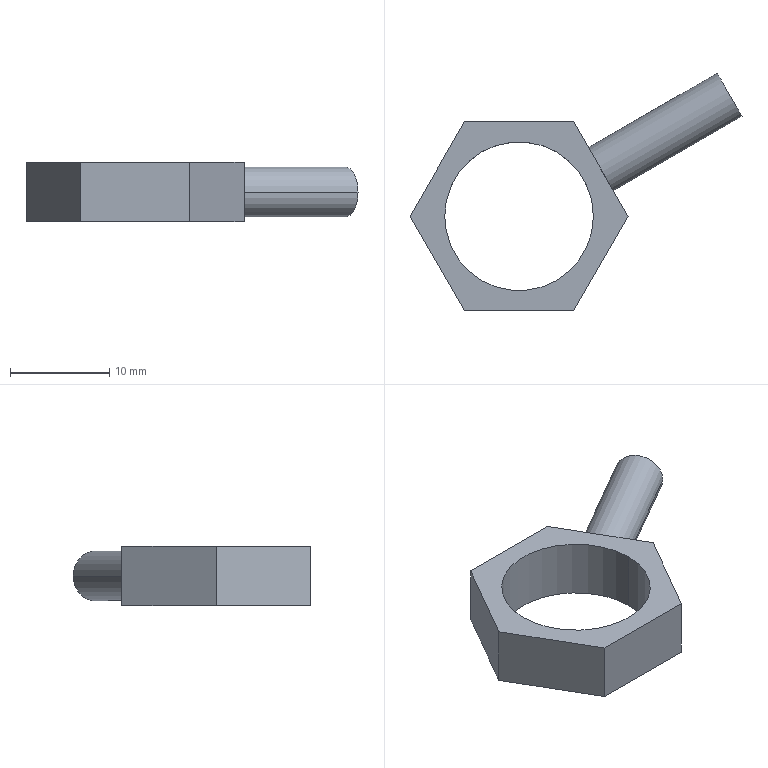Part | SolidWorks | features Extrusion 1, ICE 1 | 1 solid | 13 faces | box 33.49 x 23.954 x 6 mm | volume 1120 mm3 | plane 9 | cylinder 4 | commonest cylinder face diameters 5 x2 15 x2
STEP:
#1=CARTESIAN_POINT('',(19.99,14.428,3.));
#2=VERTEX_POINT('',#1);
#3=CARTESIAN_POINT('',(22.49,10.098,3.));
#4=VERTEX_POINT('',#3);
#5=CARTESIAN_POINT('',(21.24,12.263,3.));
#6=DIRECTION('',(0.866,0.5,0.));
#7=DIRECTION('',(-0.5,0.866,0.));
#8=AXIS2_PLACEMENT_3D('',#5,#6,#7);
#9=CIRCLE('',#8,2.5);
#10=EDGE_CURVE('',#2,#4,#9,.T.);
#11=ORIENTED_EDGE('',*,*,#10,.F.);
#12=CARTESIAN_POINT('',(7.,6.928,3.));
#13=VERTEX_POINT('',#12);
#14=CARTESIAN_POINT('',(19.99,14.428,3.));
#15=DIRECTION('',(-0.866,-0.5,0.));
#16=VECTOR('',#15,1000.);
#17=LINE('',#14,#16);
#18=EDGE_CURVE('',#2,#13,#17,.T.);
#19=ORIENTED_EDGE('',*,*,#18,.T.);
#20=CARTESIAN_POINT('',(9.5,2.598,3.));
#21=VERTEX_POINT('',#20);
#22=CARTESIAN_POINT('',(8.25,4.763,3.));
#23=DIRECTION('',(0.866,0.5,0.));
#24=DIRECTION('',(-0.5,0.866,0.));
#25=AXIS2_PLACEMENT_3D('',#22,#23,#24);
#26=CIRCLE('',#25,2.5);
#27=EDGE_CURVE('',#13,#21,#26,.T.);
#28=ORIENTED_EDGE('',*,*,#27,.T.);
#29=CARTESIAN_POINT('',(22.49,10.098,3.));
#30=DIRECTION('',(-0.866,-0.5,0.));
#31=VECTOR('',#30,1000.);
#32=LINE('',#29,#31);
#33=EDGE_CURVE('',#4,#21,#32,.T.);
#34=ORIENTED_EDGE('',*,*,#33,.F.);
#35=EDGE_LOOP('',(#11,#19,#28,#34));
#36=FACE_OUTER_BOUND('',#35,.T.);
#37=CARTESIAN_POINT('',(21.24,12.263,3.));
#38=DIRECTION('',(-0.866,-0.5,0.));
#39=DIRECTION('',(0.5,-0.866,0.));
#40=AXIS2_PLACEMENT_3D('',#37,#38,#39);
#41=CYLINDRICAL_SURFACE('',#40,2.5);
#42=ADVANCED_FACE('',(#36),#41,.T.);
#43=CARTESIAN_POINT('',(-7.5,0.,6.));
#44=VERTEX_POINT('',#43);
#45=CARTESIAN_POINT('',(7.5,0.,6.));
#46=VERTEX_POINT('',#45);
#47=CARTESIAN_POINT('',(0.,0.,6.));
#48=DIRECTION('',(0.,0.,1.));
#49=DIRECTION('',(1.,0.,0.));
#50=AXIS2_PLACEMENT_3D('',#47,#48,#49);
#51=CIRCLE('',#50,7.5);
#52=EDGE_CURVE('',#44,#46,#51,.T.);
#53=ORIENTED_EDGE('',*,*,#52,.T.);
#54=CARTESIAN_POINT('',(7.5,0.,0.));
#55=VERTEX_POINT('',#54);
#56=CARTESIAN_POINT('',(7.5,0.,6.));
#57=DIRECTION('',(0.,0.,-1.));
#58=VECTOR('',#57,1000.);
#59=LINE('',#56,#58);
#60=EDGE_CURVE('',#46,#55,#59,.T.);
#61=ORIENTED_EDGE('',*,*,#60,.T.);
#62=CARTESIAN_POINT('',(-7.5,0.,0.));
#63=VERTEX_POINT('',#62);
#64=CARTESIAN_POINT('',(0.,0.,0.));
#65=DIRECTION('',(0.,0.,1.));
#66=DIRECTION('',(1.,0.,0.));
#67=AXIS2_PLACEMENT_3D('',#64,#65,#66);
#68=CIRCLE('',#67,7.5);
#69=EDGE_CURVE('',#63,#55,#68,.T.);
#70=ORIENTED_EDGE('',*,*,#69,.F.);
#71=CARTESIAN_POINT('',(-7.5,0.,6.));
#72=DIRECTION('',(0.,0.,-1.));
#73=VECTOR('',#72,1000.);
#74=LINE('',#71,#73);
#75=EDGE_CURVE('',#44,#63,#74,.T.);
#76=ORIENTED_EDGE('',*,*,#75,.F.);
#77=EDGE_LOOP('',(#53,#61,#70,#76));
#78=FACE_OUTER_BOUND('',#77,.T.);
#79=CARTESIAN_POINT('',(0.,0.,6.));
#80=DIRECTION('',(0.,0.,-1.));
#81=DIRECTION('',(-1.,0.,0.));
#82=AXIS2_PLACEMENT_3D('',#79,#80,#81);
#83=CYLINDRICAL_SURFACE('',#82,7.5);
#84=ADVANCED_FACE('',(#78),#83,.F.);
#85=CARTESIAN_POINT('',(5.5,9.526,6.));
#86=VERTEX_POINT('',#85);
#87=CARTESIAN_POINT('',(-5.5,9.526,6.));
#88=VERTEX_POINT('',#87);
#89=CARTESIAN_POINT('',(5.5,9.526,6.));
#90=DIRECTION('',(-1.,0.,0.));
#91=VECTOR('',#90,1000.);
#92=LINE('',#89,#91);
#93=EDGE_CURVE('',#86,#88,#92,.T.);
#94=ORIENTED_EDGE('',*,*,#93,.T.);
#95=CARTESIAN_POINT('',(-11.,0.,6.));
#96=VERTEX_POINT('',#95);
#97=CARTESIAN_POINT('',(-5.5,9.526,6.));
#98=DIRECTION('',(-0.5,-0.866,0.));
#99=VECTOR('',#98,1000.);
#100=LINE('',#97,#99);
#101=EDGE_CURVE('',#88,#96,#100,.T.);
#102=ORIENTED_EDGE('',*,*,#101,.T.);
#103=CARTESIAN_POINT('',(-5.5,-9.526,6.));
#104=VERTEX_POINT('',#103);
#105=CARTESIAN_POINT('',(-11.,0.,6.));
#106=DIRECTION('',(0.5,-0.866,0.));
#107=VECTOR('',#106,1000.);
#108=LINE('',#105,#107);
#109=EDGE_CURVE('',#96,#104,#108,.T.);
#110=ORIENTED_EDGE('',*,*,#109,.T.);
#111=CARTESIAN_POINT('',(5.5,-9.526,6.));
#112=VERTEX_POINT('',#111);
#113=CARTESIAN_POINT('',(-5.5,-9.526,6.));
#114=DIRECTION('',(1.,0.,0.));
#115=VECTOR('',#114,1000.);
#116=LINE('',#113,#115);
#117=EDGE_CURVE('',#104,#112,#116,.T.);
#118=ORIENTED_EDGE('',*,*,#117,.T.);
#119=CARTESIAN_POINT('',(11.,0.,6.));
#120=VERTEX_POINT('',#119);
#121=CARTESIAN_POINT('',(5.5,-9.526,6.));
#122=DIRECTION('',(0.5,0.866,0.));
#123=VECTOR('',#122,1000.);
#124=LINE('',#121,#123);
#125=EDGE_CURVE('',#112,#120,#124,.T.);
#126=ORIENTED_EDGE('',*,*,#125,.T.);
#127=CARTESIAN_POINT('',(11.,0.,6.));
#128=DIRECTION('',(-0.5,0.866,0.));
#129=VECTOR('',#128,1000.);
#130=LINE('',#127,#129);
#131=EDGE_CURVE('',#120,#86,#130,.T.);
#132=ORIENTED_EDGE('',*,*,#131,.T.);
#133=EDGE_LOOP('',(#94,#102,#110,#118,#126,#132));
#134=FACE_OUTER_BOUND('',#133,.T.);
#135=ORIENTED_EDGE('',*,*,#52,.F.);
#136=CARTESIAN_POINT('',(0.,0.,6.));
#137=DIRECTION('',(0.,0.,1.));
#138=DIRECTION('',(1.,0.,0.));
#139=AXIS2_PLACEMENT_3D('',#136,#137,#138);
#140=CIRCLE('',#139,7.5);
#141=EDGE_CURVE('',#46,#44,#140,.T.);
#142=ORIENTED_EDGE('',*,*,#141,.F.);
#143=EDGE_LOOP('',(#135,#142));
#144=FACE_BOUND('',#143,.T.);
#145=CARTESIAN_POINT('',(0.,0.,6.));
#146=DIRECTION('',(0.,0.,1.));
#147=DIRECTION('',(1.,0.,0.));
#148=AXIS2_PLACEMENT_3D('',#145,#146,#147);
#149=PLANE('',#148);
#150=ADVANCED_FACE('',(#134,#144),#149,.T.);
#151=CARTESIAN_POINT('',(5.5,9.526,0.));
#152=VERTEX_POINT('',#151);
#153=CARTESIAN_POINT('',(-5.5,9.526,0.));
#154=VERTEX_POINT('',#153);
#155=CARTESIAN_POINT('',(5.5,9.526,0.));
#156=DIRECTION('',(-1.,0.,0.));
#157=VECTOR('',#156,1000.);
#158=LINE('',#155,#157);
#159=EDGE_CURVE('',#152,#154,#158,.T.);
#160=ORIENTED_EDGE('',*,*,#159,.F.);
#161=CARTESIAN_POINT('',(11.,0.,0.));
#162=VERTEX_POINT('',#161);
#163=CARTESIAN_POINT('',(11.,0.,0.));
#164=DIRECTION('',(-0.5,0.866,0.));
#165=VECTOR('',#164,1000.);
#166=LINE('',#163,#165);
#167=EDGE_CURVE('',#162,#152,#166,.T.);
#168=ORIENTED_EDGE('',*,*,#167,.F.);
#169=CARTESIAN_POINT('',(5.5,-9.526,0.));
#170=VERTEX_POINT('',#169);
#171=CARTESIAN_POINT('',(5.5,-9.526,0.));
#172=DIRECTION('',(0.5,0.866,0.));
#173=VECTOR('',#172,1000.);
#174=LINE('',#171,#173);
#175=EDGE_CURVE('',#170,#162,#174,.T.);
#176=ORIENTED_EDGE('',*,*,#175,.F.);
#177=CARTESIAN_POINT('',(-5.5,-9.526,0.));
#178=VERTEX_POINT('',#177);
#179=CARTESIAN_POINT('',(-5.5,-9.526,0.));
#180=DIRECTION('',(1.,0.,0.));
#181=VECTOR('',#180,1000.);
#182=LINE('',#179,#181);
#183=EDGE_CURVE('',#178,#170,#182,.T.);
#184=ORIENTED_EDGE('',*,*,#183,.F.);
#185=CARTESIAN_POINT('',(-11.,0.,0.));
#186=VERTEX_POINT('',#185);
#187=CARTESIAN_POINT('',(-11.,0.,0.));
#188=DIRECTION('',(0.5,-0.866,0.));
#189=VECTOR('',#188,1000.);
#190=LINE('',#187,#189);
#191=EDGE_CURVE('',#186,#178,#190,.T.);
#192=ORIENTED_EDGE('',*,*,#191,.F.);
#193=CARTESIAN_POINT('',(-5.5,9.526,0.));
#194=DIRECTION('',(-0.5,-0.866,0.));
#195=VECTOR('',#194,1000.);
#196=LINE('',#193,#195);
#197=EDGE_CURVE('',#154,#186,#196,.T.);
#198=ORIENTED_EDGE('',*,*,#197,.F.);
#199=EDGE_LOOP('',(#160,#168,#176,#184,#192,#198));
#200=FACE_OUTER_BOUND('',#199,.T.);
#201=ORIENTED_EDGE('',*,*,#69,.T.);
#202=CARTESIAN_POINT('',(0.,0.,0.));
#203=DIRECTION('',(0.,0.,1.));
#204=DIRECTION('',(1.,0.,0.));
#205=AXIS2_PLACEMENT_3D('',#202,#203,#204);
#206=CIRCLE('',#205,7.5);
#207=EDGE_CURVE('',#55,#63,#206,.T.);
#208=ORIENTED_EDGE('',*,*,#207,.T.);
#209=EDGE_LOOP('',(#201,#208));
#210=FACE_BOUND('',#209,.T.);
#211=CARTESIAN_POINT('',(0.,0.,0.));
#212=DIRECTION('',(0.,0.,1.));
#213=DIRECTION('',(1.,0.,0.));
#214=AXIS2_PLACEMENT_3D('',#211,#212,#213);
#215=PLANE('',#214);
#216=ADVANCED_FACE('',(#200,#210),#215,.F.);
#217=ORIENTED_EDGE('',*,*,#159,.T.);
#218=CARTESIAN_POINT('',(-5.5,9.526,6.));
#219=DIRECTION('',(0.,0.,-1.));
#220=VECTOR('',#219,1000.);
#221=LINE('',#218,#220);
#222=EDGE_CURVE('',#88,#154,#221,.T.);
#223=ORIENTED_EDGE('',*,*,#222,.F.);
#224=ORIENTED_EDGE('',*,*,#93,.F.);
#225=CARTESIAN_POINT('',(5.5,9.526,6.));
#226=DIRECTION('',(0.,0.,-1.));
#227=VECTOR('',#226,1000.);
#228=LINE('',#225,#227);
#229=EDGE_CURVE('',#86,#152,#228,.T.);
#230=ORIENTED_EDGE('',*,*,#229,.T.);
#231=EDGE_LOOP('',(#217,#223,#224,#230));
#232=FACE_OUTER_BOUND('',#231,.T.);
#233=CARTESIAN_POINT('',(5.5,9.526,6.));
#234=DIRECTION('',(0.,-1.,0.));
#235=DIRECTION('',(1.,0.,0.));
#236=AXIS2_PLACEMENT_3D('',#233,#234,#235);
#237=PLANE('',#236);
#238=ADVANCED_FACE('',(#232),#237,.F.);
#239=ORIENTED_EDGE('',*,*,#197,.T.);
#240=CARTESIAN_POINT('',(-11.,0.,6.));
#241=DIRECTION('',(0.,0.,-1.));
#242=VECTOR('',#241,1000.);
#243=LINE('',#240,#242);
#244=EDGE_CURVE('',#96,#186,#243,.T.);
#245=ORIENTED_EDGE('',*,*,#244,.F.);
#246=ORIENTED_EDGE('',*,*,#101,.F.);
#247=ORIENTED_EDGE('',*,*,#222,.T.);
#248=EDGE_LOOP('',(#239,#245,#246,#247));
#249=FACE_OUTER_BOUND('',#248,.T.);
#250=CARTESIAN_POINT('',(-5.5,9.526,6.));
#251=DIRECTION('',(0.866,-0.5,0.));
#252=DIRECTION('',(0.5,0.866,0.));
#253=AXIS2_PLACEMENT_3D('',#250,#251,#252);
#254=PLANE('',#253);
#255=ADVANCED_FACE('',(#249),#254,.F.);
#256=ORIENTED_EDGE('',*,*,#191,.T.);
#257=CARTESIAN_POINT('',(-5.5,-9.526,6.));
#258=DIRECTION('',(0.,0.,-1.));
#259=VECTOR('',#258,1000.);
#260=LINE('',#257,#259);
#261=EDGE_CURVE('',#104,#178,#260,.T.);
#262=ORIENTED_EDGE('',*,*,#261,.F.);
#263=ORIENTED_EDGE('',*,*,#109,.F.);
#264=ORIENTED_EDGE('',*,*,#244,.T.);
#265=EDGE_LOOP('',(#256,#262,#263,#264));
#266=FACE_OUTER_BOUND('',#265,.T.);
#267=CARTESIAN_POINT('',(-11.,0.,6.));
#268=DIRECTION('',(0.866,0.5,0.));
#269=DIRECTION('',(-0.5,0.866,0.));
#270=AXIS2_PLACEMENT_3D('',#267,#268,#269);
#271=PLANE('',#270);
#272=ADVANCED_FACE('',(#266),#271,.F.);
#273=ORIENTED_EDGE('',*,*,#183,.T.);
#274=CARTESIAN_POINT('',(5.5,-9.526,6.));
#275=DIRECTION('',(0.,0.,-1.));
#276=VECTOR('',#275,1000.);
#277=LINE('',#274,#276);
#278=EDGE_CURVE('',#112,#170,#277,.T.);
#279=ORIENTED_EDGE('',*,*,#278,.F.);
#280=ORIENTED_EDGE('',*,*,#117,.F.);
#281=ORIENTED_EDGE('',*,*,#261,.T.);
#282=EDGE_LOOP('',(#273,#279,#280,#281));
#283=FACE_OUTER_BOUND('',#282,.T.);
#284=CARTESIAN_POINT('',(-5.5,-9.526,6.));
#285=DIRECTION('',(0.,1.,0.));
#286=DIRECTION('',(-1.,0.,0.));
#287=AXIS2_PLACEMENT_3D('',#284,#285,#286);
#288=PLANE('',#287);
#289=ADVANCED_FACE('',(#283),#288,.F.);
#290=ORIENTED_EDGE('',*,*,#175,.T.);
#291=CARTESIAN_POINT('',(11.,0.,6.));
#292=DIRECTION('',(0.,0.,-1.));
#293=VECTOR('',#292,1000.);
#294=LINE('',#291,#293);
#295=EDGE_CURVE('',#120,#162,#294,.T.);
#296=ORIENTED_EDGE('',*,*,#295,.F.);
#297=ORIENTED_EDGE('',*,*,#125,.F.);
#298=ORIENTED_EDGE('',*,*,#278,.T.);
#299=EDGE_LOOP('',(#290,#296,#297,#298));
#300=FACE_OUTER_BOUND('',#299,.T.);
#301=CARTESIAN_POINT('',(5.5,-9.526,6.));
#302=DIRECTION('',(-0.866,0.5,0.));
#303=DIRECTION('',(-0.5,-0.866,0.));
#304=AXIS2_PLACEMENT_3D('',#301,#302,#303);
#305=PLANE('',#304);
#306=ADVANCED_FACE('',(#300),#305,.F.);
#307=CARTESIAN_POINT('',(8.25,4.763,3.));
#308=DIRECTION('',(0.866,0.5,0.));
#309=DIRECTION('',(-0.5,0.866,0.));
#310=AXIS2_PLACEMENT_3D('',#307,#308,#309);
#311=CIRCLE('',#310,2.5);
#312=EDGE_CURVE('',#21,#13,#311,.T.);
#313=ORIENTED_EDGE('',*,*,#312,.F.);
#314=ORIENTED_EDGE('',*,*,#27,.F.);
#315=EDGE_LOOP('',(#313,#314));
#316=FACE_BOUND('',#315,.T.);
#317=ORIENTED_EDGE('',*,*,#167,.T.);
#318=ORIENTED_EDGE('',*,*,#229,.F.);
#319=ORIENTED_EDGE('',*,*,#131,.F.);
#320=ORIENTED_EDGE('',*,*,#295,.T.);
#321=EDGE_LOOP('',(#317,#318,#319,#320));
#322=FACE_OUTER_BOUND('',#321,.T.);
#323=CARTESIAN_POINT('',(11.,0.,6.));
#324=DIRECTION('',(-0.866,-0.5,0.));
#325=DIRECTION('',(0.5,-0.866,0.));
#326=AXIS2_PLACEMENT_3D('',#323,#324,#325);
#327=PLANE('',#326);
#328=ADVANCED_FACE('',(#316,#322),#327,.F.);
#329=ORIENTED_EDGE('',*,*,#60,.F.);
#330=ORIENTED_EDGE('',*,*,#141,.T.);
#331=ORIENTED_EDGE('',*,*,#75,.T.);
#332=ORIENTED_EDGE('',*,*,#207,.F.);
#333=EDGE_LOOP('',(#329,#330,#331,#332));
#334=FACE_OUTER_BOUND('',#333,.T.);
#335=CARTESIAN_POINT('',(0.,0.,6.));
#336=DIRECTION('',(0.,0.,-1.));
#337=DIRECTION('',(-1.,0.,0.));
#338=AXIS2_PLACEMENT_3D('',#335,#336,#337);
#339=CYLINDRICAL_SURFACE('',#338,7.5);
#340=ADVANCED_FACE('',(#334),#339,.F.);
#341=ORIENTED_EDGE('',*,*,#18,.F.);
#342=CARTESIAN_POINT('',(21.24,12.263,3.));
#343=DIRECTION('',(0.866,0.5,0.));
#344=DIRECTION('',(-0.5,0.866,0.));
#345=AXIS2_PLACEMENT_3D('',#342,#343,#344);
#346=CIRCLE('',#345,2.5);
#347=EDGE_CURVE('',#4,#2,#346,.T.);
#348=ORIENTED_EDGE('',*,*,#347,.F.);
#349=ORIENTED_EDGE('',*,*,#33,.T.);
#350=ORIENTED_EDGE('',*,*,#312,.T.);
#351=EDGE_LOOP('',(#341,#348,#349,#350));
#352=FACE_OUTER_BOUND('',#351,.T.);
#353=CARTESIAN_POINT('',(21.24,12.263,3.));
#354=DIRECTION('',(-0.866,-0.5,0.));
#355=DIRECTION('',(0.5,-0.866,0.));
#356=AXIS2_PLACEMENT_3D('',#353,#354,#355);
#357=CYLINDRICAL_SURFACE('',#356,2.5);
#358=ADVANCED_FACE('',(#352),#357,.T.);
#359=ORIENTED_EDGE('',*,*,#347,.T.);
#360=ORIENTED_EDGE('',*,*,#10,.T.);
#361=EDGE_LOOP('',(#359,#360));
#362=FACE_OUTER_BOUND('',#361,.T.);
#363=CARTESIAN_POINT('',(21.24,12.263,3.));
#364=DIRECTION('',(0.866,0.5,0.));
#365=DIRECTION('',(-0.5,0.866,0.));
#366=AXIS2_PLACEMENT_3D('',#363,#364,#365);
#367=PLANE('',#366);
#368=ADVANCED_FACE('',(#362),#367,.T.);
#369=CLOSED_SHELL('',(#42,#84,#150,#216,#238,#255,#272,#289,#306,#328,#340,#358,#368));
#370=MANIFOLD_SOLID_BREP('',#369);
#371=CARTESIAN_POINT('',(0.,0.,0.));
#372=DIRECTION('',(0.,0.,1.));
#373=DIRECTION('',(1.,0.,0.));
#374=AXIS2_PLACEMENT_3D('',#371,#372,#373);
#375=(LENGTH_UNIT()NAMED_UNIT(*)SI_UNIT(.MILLI.,.METRE.));
#376=UNCERTAINTY_MEASURE_WITH_UNIT(LENGTH_MEASURE(0.00001),#375,'','');
#377=(NAMED_UNIT(*)PLANE_ANGLE_UNIT()SI_UNIT($,.RADIAN.));
#378=(NAMED_UNIT(*)SI_UNIT($,.STERADIAN.)SOLID_ANGLE_UNIT());
#379=(GEOMETRIC_REPRESENTATION_CONTEXT(3)GLOBAL_UNCERTAINTY_ASSIGNED_CONTEXT((#376))GLOBAL_UNIT_ASSIGNED_CONTEXT((#375,#377,#378))REPRESENTATION_CONTEXT('',''));
#380=ADVANCED_BREP_SHAPE_REPRESENTATION('',(#370,#374),#379);